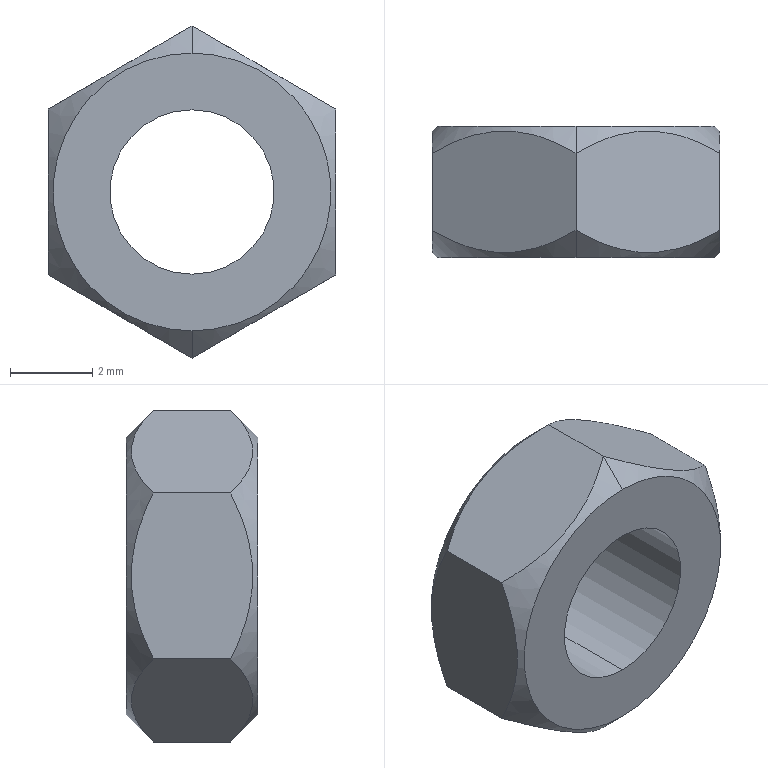Part | SolidWorks | features Extrusion 1, ICE 1, RevCut 1 | 1 solid | 14 faces | box 7 x 3.2 x 8.083 mm | volume 93.048 mm3 | plane 8 | cone 4 | cylinder 2 | commonest cylinder face diameters 4 x2
STEP:
#1=CARTESIAN_POINT('',(0.,0.,-2.));
#2=VERTEX_POINT('',#1);
#3=CARTESIAN_POINT('',(0.,0.,2.));
#4=VERTEX_POINT('',#3);
#5=CARTESIAN_POINT('',(0.,0.,0.));
#6=DIRECTION('',(0.,1.,0.));
#7=DIRECTION('',(0.,0.,1.));
#8=AXIS2_PLACEMENT_3D('',#5,#6,#7);
#9=CIRCLE('',#8,2.);
#10=EDGE_CURVE('',#2,#4,#9,.T.);
#11=ORIENTED_EDGE('',*,*,#10,.F.);
#12=CARTESIAN_POINT('',(0.,3.2,-2.));
#13=VERTEX_POINT('',#12);
#14=CARTESIAN_POINT('',(0.,0.,-2.));
#15=DIRECTION('',(0.,1.,0.));
#16=VECTOR('',#15,1000.);
#17=LINE('',#14,#16);
#18=EDGE_CURVE('',#2,#13,#17,.T.);
#19=ORIENTED_EDGE('',*,*,#18,.T.);
#20=CARTESIAN_POINT('',(0.,3.2,2.));
#21=VERTEX_POINT('',#20);
#22=CARTESIAN_POINT('',(0.,3.2,0.));
#23=DIRECTION('',(0.,1.,0.));
#24=DIRECTION('',(0.,0.,1.));
#25=AXIS2_PLACEMENT_3D('',#22,#23,#24);
#26=CIRCLE('',#25,2.);
#27=EDGE_CURVE('',#13,#21,#26,.T.);
#28=ORIENTED_EDGE('',*,*,#27,.T.);
#29=CARTESIAN_POINT('',(0.,0.,2.));
#30=DIRECTION('',(0.,1.,0.));
#31=VECTOR('',#30,1000.);
#32=LINE('',#29,#31);
#33=EDGE_CURVE('',#4,#21,#32,.T.);
#34=ORIENTED_EDGE('',*,*,#33,.F.);
#35=EDGE_LOOP('',(#11,#19,#28,#34));
#36=FACE_OUTER_BOUND('',#35,.T.);
#37=CARTESIAN_POINT('',(0.,0.,0.));
#38=DIRECTION('',(0.,1.,0.));
#39=DIRECTION('',(0.,0.,1.));
#40=AXIS2_PLACEMENT_3D('',#37,#38,#39);
#41=CYLINDRICAL_SURFACE('',#40,2.);
#42=ADVANCED_FACE('',(#36),#41,.F.);
#43=CARTESIAN_POINT('',(0.,3.2,-3.381));
#44=VERTEX_POINT('',#43);
#45=CARTESIAN_POINT('',(0.,3.2,3.381));
#46=VERTEX_POINT('',#45);
#47=CARTESIAN_POINT('',(0.,3.2,0.));
#48=DIRECTION('',(0.,-1.,0.));
#49=DIRECTION('',(0.,0.,-1.));
#50=AXIS2_PLACEMENT_3D('',#47,#48,#49);
#51=CIRCLE('',#50,3.381);
#52=EDGE_CURVE('',#44,#46,#51,.T.);
#53=ORIENTED_EDGE('',*,*,#52,.T.);
#54=CARTESIAN_POINT('',(0.,2.54,4.041));
#55=VERTEX_POINT('',#54);
#56=CARTESIAN_POINT('',(0.,3.2,3.381));
#57=DIRECTION('',(0.,-0.7071,0.7071));
#58=VECTOR('',#57,1000.);
#59=LINE('',#56,#58);
#60=EDGE_CURVE('',#46,#55,#59,.T.);
#61=ORIENTED_EDGE('',*,*,#60,.T.);
#62=CARTESIAN_POINT('',(3.5,2.54,2.021));
#63=VERTEX_POINT('',#62);
#64=CARTESIAN_POINT('',(3.5,2.54,2.021));
#65=CARTESIAN_POINT('',(3.227,2.698,2.179));
#66=CARTESIAN_POINT('',(2.947,2.832,2.34));
#67=CARTESIAN_POINT('',(2.512,2.976,2.591));
#68=CARTESIAN_POINT('',(2.365,3.014,2.676));
#69=CARTESIAN_POINT('',(2.064,3.067,2.85));
#70=CARTESIAN_POINT('',(1.909,3.081,2.939));
#71=CARTESIAN_POINT('',(1.451,3.082,3.204));
#72=CARTESIAN_POINT('',(1.151,3.029,3.377));
#73=CARTESIAN_POINT('',(0.5583,2.835,3.719));
#74=CARTESIAN_POINT('',(0.2751,2.699,3.883));
#75=CARTESIAN_POINT('',(0.,2.54,4.041));
#76=B_SPLINE_CURVE_WITH_KNOTS('',3,(#64,#65,#66,#67,#68,#69,#70,#71,#72,#73,#74,#75),.UNSPECIFIED.,.F.,.F.,(4,2,2,2,2,4),(0.000000254,0.001044,0.001566,0.002088,0.003131,0.004175),.UNSPECIFIED.);
#77=EDGE_CURVE('',#63,#55,#76,.T.);
#78=ORIENTED_EDGE('',*,*,#77,.F.);
#79=CARTESIAN_POINT('',(3.5,2.54,-2.021));
#80=VERTEX_POINT('',#79);
#81=CARTESIAN_POINT('',(3.5,2.54,-2.021));
#82=CARTESIAN_POINT('',(3.5,2.618,-1.864));
#83=CARTESIAN_POINT('',(3.5,2.691,-1.705));
#84=CARTESIAN_POINT('',(3.5,2.823,-1.378));
#85=CARTESIAN_POINT('',(3.5,2.882,-1.21));
#86=CARTESIAN_POINT('',(3.5,3.026,-0.7022));
#87=CARTESIAN_POINT('',(3.5,3.081,-0.357));
#88=CARTESIAN_POINT('',(3.5,3.082,0.1745));
#89=CARTESIAN_POINT('',(3.5,3.068,0.3526));
#90=CARTESIAN_POINT('',(3.5,3.016,0.7001));
#91=CARTESIAN_POINT('',(3.5,2.978,0.871));
#92=CARTESIAN_POINT('',(3.5,2.834,1.377));
#93=CARTESIAN_POINT('',(3.5,2.697,1.707));
#94=CARTESIAN_POINT('',(3.5,2.54,2.021));
#95=B_SPLINE_CURVE_WITH_KNOTS('',3,(#81,#82,#83,#84,#85,#86,#87,#88,#89,#90,#91,#92,#93,#94),.UNSPECIFIED.,.F.,.F.,(4,2,2,2,2,2,4),(0.005098,0.005624,0.00615,0.007203,0.00773,0.008256,0.009309),.UNSPECIFIED.);
#96=EDGE_CURVE('',#80,#63,#95,.T.);
#97=ORIENTED_EDGE('',*,*,#96,.F.);
#98=CARTESIAN_POINT('',(0.,2.54,-4.041));
#99=VERTEX_POINT('',#98);
#100=CARTESIAN_POINT('',(0.,2.54,-4.041));
#101=CARTESIAN_POINT('',(0.2735,2.698,-3.884));
#102=CARTESIAN_POINT('',(0.5531,2.832,-3.722));
#103=CARTESIAN_POINT('',(0.9875,2.976,-3.471));
#104=CARTESIAN_POINT('',(1.135,3.014,-3.386));
#105=CARTESIAN_POINT('',(1.436,3.067,-3.212));
#106=CARTESIAN_POINT('',(1.591,3.081,-3.123));
#107=CARTESIAN_POINT('',(2.049,3.082,-2.858));
#108=CARTESIAN_POINT('',(2.349,3.029,-2.685));
#109=CARTESIAN_POINT('',(2.942,2.835,-2.343));
#110=CARTESIAN_POINT('',(3.225,2.699,-2.18));
#111=CARTESIAN_POINT('',(3.5,2.54,-2.021));
#112=B_SPLINE_CURVE_WITH_KNOTS('',3,(#100,#101,#102,#103,#104,#105,#106,#107,#108,#109,#110,#111),.UNSPECIFIED.,.F.,.F.,(4,2,2,2,2,4),(0.000000254,0.001044,0.001566,0.002088,0.003131,0.004175),.UNSPECIFIED.);
#113=EDGE_CURVE('',#99,#80,#112,.T.);
#114=ORIENTED_EDGE('',*,*,#113,.F.);
#115=CARTESIAN_POINT('',(0.,3.2,-3.381));
#116=DIRECTION('',(0.,-0.7071,-0.7071));
#117=VECTOR('',#116,1000.);
#118=LINE('',#115,#117);
#119=EDGE_CURVE('',#44,#99,#118,.T.);
#120=ORIENTED_EDGE('',*,*,#119,.F.);
#121=EDGE_LOOP('',(#53,#61,#78,#97,#114,#120));
#122=FACE_OUTER_BOUND('',#121,.T.);
#123=CARTESIAN_POINT('',(0.,3.2,0.));
#124=DIRECTION('',(0.,-1.,0.));
#125=DIRECTION('',(0.,0.,-1.));
#126=AXIS2_PLACEMENT_3D('',#123,#124,#125);
#127=CONICAL_SURFACE('',#126,3.381,0.7854);
#128=ADVANCED_FACE('',(#122),#127,.T.);
#129=CARTESIAN_POINT('',(0.,0.,-3.381));
#130=VERTEX_POINT('',#129);
#131=CARTESIAN_POINT('',(0.,0.,3.381));
#132=VERTEX_POINT('',#131);
#133=CARTESIAN_POINT('',(0.,0.,0.));
#134=DIRECTION('',(0.,-1.,0.));
#135=DIRECTION('',(0.,0.,-1.));
#136=AXIS2_PLACEMENT_3D('',#133,#134,#135);
#137=CIRCLE('',#136,3.381);
#138=EDGE_CURVE('',#130,#132,#137,.T.);
#139=ORIENTED_EDGE('',*,*,#138,.F.);
#140=CARTESIAN_POINT('',(0.,0.66,-4.041));
#141=VERTEX_POINT('',#140);
#142=CARTESIAN_POINT('',(0.,0.66,-4.041));
#143=DIRECTION('',(0.,0.7071,-0.7071));
#144=VECTOR('',#143,1000.);
#145=LINE('',#142,#144);
#146=EDGE_CURVE('',#130,#141,#145,.T.);
#147=ORIENTED_EDGE('',*,*,#146,.T.);
#148=CARTESIAN_POINT('',(3.5,0.66,-2.021));
#149=VERTEX_POINT('',#148);
#150=CARTESIAN_POINT('',(3.5,0.66,-2.021));
#151=CARTESIAN_POINT('',(3.227,0.5021,-2.179));
#152=CARTESIAN_POINT('',(2.947,0.3679,-2.34));
#153=CARTESIAN_POINT('',(2.512,0.224,-2.591));
#154=CARTESIAN_POINT('',(2.365,0.1858,-2.676));
#155=CARTESIAN_POINT('',(2.064,0.1331,-2.85));
#156=CARTESIAN_POINT('',(1.909,0.1189,-2.939));
#157=CARTESIAN_POINT('',(1.451,0.1178,-3.204));
#158=CARTESIAN_POINT('',(1.151,0.1712,-3.377));
#159=CARTESIAN_POINT('',(0.5583,0.365,-3.719));
#160=CARTESIAN_POINT('',(0.2751,0.5012,-3.883));
#161=CARTESIAN_POINT('',(0.,0.66,-4.041));
#162=B_SPLINE_CURVE_WITH_KNOTS('',3,(#150,#151,#152,#153,#154,#155,#156,#157,#158,#159,#160,#161),.UNSPECIFIED.,.F.,.F.,(4,2,2,2,2,4),(0.000000254,0.001044,0.001566,0.002088,0.003131,0.004175),.UNSPECIFIED.);
#163=EDGE_CURVE('',#149,#141,#162,.T.);
#164=ORIENTED_EDGE('',*,*,#163,.F.);
#165=CARTESIAN_POINT('',(3.5,0.66,2.021));
#166=VERTEX_POINT('',#165);
#167=CARTESIAN_POINT('',(3.5,0.66,2.021));
#168=CARTESIAN_POINT('',(3.5,0.5818,1.864));
#169=CARTESIAN_POINT('',(3.5,0.5088,1.705));
#170=CARTESIAN_POINT('',(3.5,0.377,1.378));
#171=CARTESIAN_POINT('',(3.5,0.3181,1.21));
#172=CARTESIAN_POINT('',(3.5,0.1735,0.7022));
#173=CARTESIAN_POINT('',(3.5,0.1188,0.357));
#174=CARTESIAN_POINT('',(3.5,0.1184,-0.1745));
#175=CARTESIAN_POINT('',(3.5,0.1321,-0.3526));
#176=CARTESIAN_POINT('',(3.5,0.1837,-0.7001));
#177=CARTESIAN_POINT('',(3.5,0.2217,-0.871));
#178=CARTESIAN_POINT('',(3.5,0.3657,-1.377));
#179=CARTESIAN_POINT('',(3.5,0.5031,-1.707));
#180=CARTESIAN_POINT('',(3.5,0.66,-2.021));
#181=B_SPLINE_CURVE_WITH_KNOTS('',3,(#167,#168,#169,#170,#171,#172,#173,#174,#175,#176,#177,#178,#179,#180),.UNSPECIFIED.,.F.,.F.,(4,2,2,2,2,2,4),(0.005098,0.005624,0.00615,0.007203,0.00773,0.008256,0.009309),.UNSPECIFIED.);
#182=EDGE_CURVE('',#166,#149,#181,.T.);
#183=ORIENTED_EDGE('',*,*,#182,.F.);
#184=CARTESIAN_POINT('',(0.,0.66,4.041));
#185=VERTEX_POINT('',#184);
#186=CARTESIAN_POINT('',(0.,0.66,4.041));
#187=CARTESIAN_POINT('',(0.2735,0.5021,3.884));
#188=CARTESIAN_POINT('',(0.5531,0.3679,3.722));
#189=CARTESIAN_POINT('',(0.9875,0.224,3.471));
#190=CARTESIAN_POINT('',(1.135,0.1858,3.386));
#191=CARTESIAN_POINT('',(1.436,0.1331,3.212));
#192=CARTESIAN_POINT('',(1.591,0.1189,3.123));
#193=CARTESIAN_POINT('',(2.049,0.1178,2.858));
#194=CARTESIAN_POINT('',(2.349,0.1712,2.685));
#195=CARTESIAN_POINT('',(2.942,0.365,2.343));
#196=CARTESIAN_POINT('',(3.225,0.5012,2.18));
#197=CARTESIAN_POINT('',(3.5,0.66,2.021));
#198=B_SPLINE_CURVE_WITH_KNOTS('',3,(#186,#187,#188,#189,#190,#191,#192,#193,#194,#195,#196,#197),.UNSPECIFIED.,.F.,.F.,(4,2,2,2,2,4),(0.000000254,0.001044,0.001566,0.002088,0.003131,0.004175),.UNSPECIFIED.);
#199=EDGE_CURVE('',#185,#166,#198,.T.);
#200=ORIENTED_EDGE('',*,*,#199,.F.);
#201=CARTESIAN_POINT('',(0.,0.66,4.041));
#202=DIRECTION('',(0.,0.7071,0.7071));
#203=VECTOR('',#202,1000.);
#204=LINE('',#201,#203);
#205=EDGE_CURVE('',#132,#185,#204,.T.);
#206=ORIENTED_EDGE('',*,*,#205,.F.);
#207=EDGE_LOOP('',(#139,#147,#164,#183,#200,#206));
#208=FACE_OUTER_BOUND('',#207,.T.);
#209=CARTESIAN_POINT('',(0.,0.66,0.));
#210=DIRECTION('',(0.,1.,0.));
#211=DIRECTION('',(0.,0.,1.));
#212=AXIS2_PLACEMENT_3D('',#209,#210,#211);
#213=CONICAL_SURFACE('',#212,4.041,0.7854);
#214=ADVANCED_FACE('',(#208),#213,.T.);
#215=CARTESIAN_POINT('',(0.,0.,0.));
#216=DIRECTION('',(0.,1.,0.));
#217=DIRECTION('',(0.,0.,1.));
#218=AXIS2_PLACEMENT_3D('',#215,#216,#217);
#219=CIRCLE('',#218,2.);
#220=EDGE_CURVE('',#4,#2,#219,.T.);
#221=ORIENTED_EDGE('',*,*,#220,.T.);
#222=ORIENTED_EDGE('',*,*,#10,.T.);
#223=EDGE_LOOP('',(#221,#222));
#224=FACE_BOUND('',#223,.T.);
#225=CARTESIAN_POINT('',(0.,0.,0.));
#226=DIRECTION('',(0.,-1.,0.));
#227=DIRECTION('',(0.,0.,-1.));
#228=AXIS2_PLACEMENT_3D('',#225,#226,#227);
#229=CIRCLE('',#228,3.381);
#230=EDGE_CURVE('',#132,#130,#229,.T.);
#231=ORIENTED_EDGE('',*,*,#230,.T.);
#232=ORIENTED_EDGE('',*,*,#138,.T.);
#233=EDGE_LOOP('',(#231,#232));
#234=FACE_OUTER_BOUND('',#233,.T.);
#235=CARTESIAN_POINT('',(0.,0.,0.));
#236=DIRECTION('',(0.,1.,0.));
#237=DIRECTION('',(0.,0.,1.));
#238=AXIS2_PLACEMENT_3D('',#235,#236,#237);
#239=PLANE('',#238);
#240=ADVANCED_FACE('',(#224,#234),#239,.F.);
#241=ORIENTED_EDGE('',*,*,#146,.F.);
#242=ORIENTED_EDGE('',*,*,#230,.F.);
#243=ORIENTED_EDGE('',*,*,#205,.T.);
#244=CARTESIAN_POINT('',(-3.5,0.66,2.021));
#245=VERTEX_POINT('',#244);
#246=CARTESIAN_POINT('',(-3.5,0.66,2.021));
#247=CARTESIAN_POINT('',(-3.227,0.5021,2.179));
#248=CARTESIAN_POINT('',(-2.947,0.3679,2.34));
#249=CARTESIAN_POINT('',(-2.512,0.224,2.591));
#250=CARTESIAN_POINT('',(-2.365,0.1858,2.676));
#251=CARTESIAN_POINT('',(-2.064,0.1331,2.85));
#252=CARTESIAN_POINT('',(-1.909,0.1189,2.939));
#253=CARTESIAN_POINT('',(-1.451,0.1178,3.204));
#254=CARTESIAN_POINT('',(-1.151,0.1712,3.377));
#255=CARTESIAN_POINT('',(-0.5583,0.365,3.719));
#256=CARTESIAN_POINT('',(-0.2751,0.5012,3.883));
#257=CARTESIAN_POINT('',(0.,0.66,4.041));
#258=B_SPLINE_CURVE_WITH_KNOTS('',3,(#246,#247,#248,#249,#250,#251,#252,#253,#254,#255,#256,#257),.UNSPECIFIED.,.F.,.F.,(4,2,2,2,2,4),(0.000000254,0.001044,0.001566,0.002088,0.003131,0.004175),.UNSPECIFIED.);
#259=EDGE_CURVE('',#245,#185,#258,.T.);
#260=ORIENTED_EDGE('',*,*,#259,.F.);
#261=CARTESIAN_POINT('',(-3.5,0.66,-2.021));
#262=VERTEX_POINT('',#261);
#263=CARTESIAN_POINT('',(-3.5,0.66,-2.021));
#264=CARTESIAN_POINT('',(-3.5,0.5818,-1.864));
#265=CARTESIAN_POINT('',(-3.5,0.5088,-1.705));
#266=CARTESIAN_POINT('',(-3.5,0.377,-1.378));
#267=CARTESIAN_POINT('',(-3.5,0.3181,-1.21));
#268=CARTESIAN_POINT('',(-3.5,0.1735,-0.7022));
#269=CARTESIAN_POINT('',(-3.5,0.1188,-0.357));
#270=CARTESIAN_POINT('',(-3.5,0.1184,0.1745));
#271=CARTESIAN_POINT('',(-3.5,0.1321,0.3526));
#272=CARTESIAN_POINT('',(-3.5,0.1837,0.7001));
#273=CARTESIAN_POINT('',(-3.5,0.2217,0.871));
#274=CARTESIAN_POINT('',(-3.5,0.3657,1.377));
#275=CARTESIAN_POINT('',(-3.5,0.5031,1.707));
#276=CARTESIAN_POINT('',(-3.5,0.66,2.021));
#277=B_SPLINE_CURVE_WITH_KNOTS('',3,(#263,#264,#265,#266,#267,#268,#269,#270,#271,#272,#273,#274,#275,#276),.UNSPECIFIED.,.F.,.F.,(4,2,2,2,2,2,4),(0.005098,0.005624,0.00615,0.007203,0.00773,0.008256,0.009309),.UNSPECIFIED.);
#278=EDGE_CURVE('',#262,#245,#277,.T.);
#279=ORIENTED_EDGE('',*,*,#278,.F.);
#280=CARTESIAN_POINT('',(0.,0.66,-4.041));
#281=CARTESIAN_POINT('',(-0.2735,0.5021,-3.884));
#282=CARTESIAN_POINT('',(-0.5531,0.3679,-3.722));
#283=CARTESIAN_POINT('',(-0.9875,0.224,-3.471));
#284=CARTESIAN_POINT('',(-1.135,0.1858,-3.386));
#285=CARTESIAN_POINT('',(-1.436,0.1331,-3.212));
#286=CARTESIAN_POINT('',(-1.591,0.1189,-3.123));
#287=CARTESIAN_POINT('',(-2.049,0.1178,-2.858));
#288=CARTESIAN_POINT('',(-2.349,0.1712,-2.685));
#289=CARTESIAN_POINT('',(-2.942,0.365,-2.343));
#290=CARTESIAN_POINT('',(-3.225,0.5012,-2.18));
#291=CARTESIAN_POINT('',(-3.5,0.66,-2.021));
#292=B_SPLINE_CURVE_WITH_KNOTS('',3,(#280,#281,#282,#283,#284,#285,#286,#287,#288,#289,#290,#291),.UNSPECIFIED.,.F.,.F.,(4,2,2,2,2,4),(0.000000254,0.001044,0.001566,0.002088,0.003131,0.004175),.UNSPECIFIED.);
#293=EDGE_CURVE('',#141,#262,#292,.T.);
#294=ORIENTED_EDGE('',*,*,#293,.F.);
#295=EDGE_LOOP('',(#241,#242,#243,#260,#279,#294));
#296=FACE_OUTER_BOUND('',#295,.T.);
#297=CARTESIAN_POINT('',(0.,0.66,0.));
#298=DIRECTION('',(0.,1.,0.));
#299=DIRECTION('',(0.,0.,1.));
#300=AXIS2_PLACEMENT_3D('',#297,#298,#299);
#301=CONICAL_SURFACE('',#300,4.041,0.7854);
#302=ADVANCED_FACE('',(#296),#301,.T.);
#303=CARTESIAN_POINT('',(0.,3.2,-4.041));
#304=DIRECTION('',(0.,-1.,0.));
#305=VECTOR('',#304,1000.);
#306=LINE('',#303,#305);
#307=EDGE_CURVE('',#99,#141,#306,.T.);
#308=ORIENTED_EDGE('',*,*,#307,.F.);
#309=ORIENTED_EDGE('',*,*,#113,.T.);
#310=CARTESIAN_POINT('',(3.5,3.2,-2.021));
#311=DIRECTION('',(0.,-1.,0.));
#312=VECTOR('',#311,1000.);
#313=LINE('',#310,#312);
#314=EDGE_CURVE('',#80,#149,#313,.T.);
#315=ORIENTED_EDGE('',*,*,#314,.T.);
#316=ORIENTED_EDGE('',*,*,#163,.T.);
#317=EDGE_LOOP('',(#308,#309,#315,#316));
#318=FACE_OUTER_BOUND('',#317,.T.);
#319=CARTESIAN_POINT('',(3.5,3.2,-2.021));
#320=DIRECTION('',(-0.5,0.,0.866));
#321=DIRECTION('',(0.866,0.,0.5));
#322=AXIS2_PLACEMENT_3D('',#319,#320,#321);
#323=PLANE('',#322);
#324=ADVANCED_FACE('',(#318),#323,.F.);
#325=CARTESIAN_POINT('',(-3.5,2.54,-2.021));
#326=VERTEX_POINT('',#325);
#327=CARTESIAN_POINT('',(-3.5,3.2,-2.021));
#328=DIRECTION('',(0.,-1.,0.));
#329=VECTOR('',#328,1000.);
#330=LINE('',#327,#329);
#331=EDGE_CURVE('',#326,#262,#330,.T.);
#332=ORIENTED_EDGE('',*,*,#331,.F.);
#333=CARTESIAN_POINT('',(-3.5,2.54,-2.021));
#334=CARTESIAN_POINT('',(-3.227,2.698,-2.179));
#335=CARTESIAN_POINT('',(-2.947,2.832,-2.34));
#336=CARTESIAN_POINT('',(-2.512,2.976,-2.591));
#337=CARTESIAN_POINT('',(-2.365,3.014,-2.676));
#338=CARTESIAN_POINT('',(-2.064,3.067,-2.85));
#339=CARTESIAN_POINT('',(-1.909,3.081,-2.939));
#340=CARTESIAN_POINT('',(-1.451,3.082,-3.204));
#341=CARTESIAN_POINT('',(-1.151,3.029,-3.377));
#342=CARTESIAN_POINT('',(-0.5583,2.835,-3.719));
#343=CARTESIAN_POINT('',(-0.2751,2.699,-3.883));
#344=CARTESIAN_POINT('',(0.,2.54,-4.041));
#345=B_SPLINE_CURVE_WITH_KNOTS('',3,(#333,#334,#335,#336,#337,#338,#339,#340,#341,#342,#343,#344),.UNSPECIFIED.,.F.,.F.,(4,2,2,2,2,4),(0.000000254,0.001044,0.001566,0.002088,0.003131,0.004175),.UNSPECIFIED.);
#346=EDGE_CURVE('',#326,#99,#345,.T.);
#347=ORIENTED_EDGE('',*,*,#346,.T.);
#348=ORIENTED_EDGE('',*,*,#307,.T.);
#349=ORIENTED_EDGE('',*,*,#293,.T.);
#350=EDGE_LOOP('',(#332,#347,#348,#349));
#351=FACE_OUTER_BOUND('',#350,.T.);
#352=CARTESIAN_POINT('',(0.,3.2,-4.041));
#353=DIRECTION('',(0.5,0.,0.866));
#354=DIRECTION('',(0.866,0.,-0.5));
#355=AXIS2_PLACEMENT_3D('',#352,#353,#354);
#356=PLANE('',#355);
#357=ADVANCED_FACE('',(#351),#356,.F.);
#358=CARTESIAN_POINT('',(-3.5,2.54,2.021));
#359=VERTEX_POINT('',#358);
#360=CARTESIAN_POINT('',(-3.5,3.2,2.021));
#361=DIRECTION('',(0.,-1.,0.));
#362=VECTOR('',#361,1000.);
#363=LINE('',#360,#362);
#364=EDGE_CURVE('',#359,#245,#363,.T.);
#365=ORIENTED_EDGE('',*,*,#364,.F.);
#366=CARTESIAN_POINT('',(-3.5,2.54,2.021));
#367=CARTESIAN_POINT('',(-3.5,2.618,1.864));
#368=CARTESIAN_POINT('',(-3.5,2.691,1.705));
#369=CARTESIAN_POINT('',(-3.5,2.823,1.378));
#370=CARTESIAN_POINT('',(-3.5,2.882,1.21));
#371=CARTESIAN_POINT('',(-3.5,3.026,0.7022));
#372=CARTESIAN_POINT('',(-3.5,3.081,0.357));
#373=CARTESIAN_POINT('',(-3.5,3.082,-0.1745));
#374=CARTESIAN_POINT('',(-3.5,3.068,-0.3526));
#375=CARTESIAN_POINT('',(-3.5,3.016,-0.7001));
#376=CARTESIAN_POINT('',(-3.5,2.978,-0.871));
#377=CARTESIAN_POINT('',(-3.5,2.834,-1.377));
#378=CARTESIAN_POINT('',(-3.5,2.697,-1.707));
#379=CARTESIAN_POINT('',(-3.5,2.54,-2.021));
#380=B_SPLINE_CURVE_WITH_KNOTS('',3,(#366,#367,#368,#369,#370,#371,#372,#373,#374,#375,#376,#377,#378,#379),.UNSPECIFIED.,.F.,.F.,(4,2,2,2,2,2,4),(0.005098,0.005624,0.00615,0.007203,0.00773,0.008256,0.009309),.UNSPECIFIED.);
#381=EDGE_CURVE('',#359,#326,#380,.T.);
#382=ORIENTED_EDGE('',*,*,#381,.T.);
#383=ORIENTED_EDGE('',*,*,#331,.T.);
#384=ORIENTED_EDGE('',*,*,#278,.T.);
#385=EDGE_LOOP('',(#365,#382,#383,#384));
#386=FACE_OUTER_BOUND('',#385,.T.);
#387=CARTESIAN_POINT('',(-3.5,3.2,-2.021));
#388=DIRECTION('',(1.,0.,0.));
#389=DIRECTION('',(0.,0.,-1.));
#390=AXIS2_PLACEMENT_3D('',#387,#388,#389);
#391=PLANE('',#390);
#392=ADVANCED_FACE('',(#386),#391,.F.);
#393=CARTESIAN_POINT('',(0.,3.2,4.041));
#394=DIRECTION('',(0.,-1.,0.));
#395=VECTOR('',#394,1000.);
#396=LINE('',#393,#395);
#397=EDGE_CURVE('',#55,#185,#396,.T.);
#398=ORIENTED_EDGE('',*,*,#397,.F.);
#399=CARTESIAN_POINT('',(0.,2.54,4.041));
#400=CARTESIAN_POINT('',(-0.2735,2.698,3.884));
#401=CARTESIAN_POINT('',(-0.5531,2.832,3.722));
#402=CARTESIAN_POINT('',(-0.9875,2.976,3.471));
#403=CARTESIAN_POINT('',(-1.135,3.014,3.386));
#404=CARTESIAN_POINT('',(-1.436,3.067,3.212));
#405=CARTESIAN_POINT('',(-1.591,3.081,3.123));
#406=CARTESIAN_POINT('',(-2.049,3.082,2.858));
#407=CARTESIAN_POINT('',(-2.349,3.029,2.685));
#408=CARTESIAN_POINT('',(-2.942,2.835,2.343));
#409=CARTESIAN_POINT('',(-3.225,2.699,2.18));
#410=CARTESIAN_POINT('',(-3.5,2.54,2.021));
#411=B_SPLINE_CURVE_WITH_KNOTS('',3,(#399,#400,#401,#402,#403,#404,#405,#406,#407,#408,#409,#410),.UNSPECIFIED.,.F.,.F.,(4,2,2,2,2,4),(0.000000254,0.001044,0.001566,0.002088,0.003131,0.004175),.UNSPECIFIED.);
#412=EDGE_CURVE('',#55,#359,#411,.T.);
#413=ORIENTED_EDGE('',*,*,#412,.T.);
#414=ORIENTED_EDGE('',*,*,#364,.T.);
#415=ORIENTED_EDGE('',*,*,#259,.T.);
#416=EDGE_LOOP('',(#398,#413,#414,#415));
#417=FACE_OUTER_BOUND('',#416,.T.);
#418=CARTESIAN_POINT('',(-3.5,3.2,2.021));
#419=DIRECTION('',(0.5,0.,-0.866));
#420=DIRECTION('',(-0.866,0.,-0.5));
#421=AXIS2_PLACEMENT_3D('',#418,#419,#420);
#422=PLANE('',#421);
#423=ADVANCED_FACE('',(#417),#422,.F.);
#424=CARTESIAN_POINT('',(3.5,3.2,2.021));
#425=DIRECTION('',(0.,-1.,0.));
#426=VECTOR('',#425,1000.);
#427=LINE('',#424,#426);
#428=EDGE_CURVE('',#63,#166,#427,.T.);
#429=ORIENTED_EDGE('',*,*,#428,.F.);
#430=ORIENTED_EDGE('',*,*,#77,.T.);
#431=ORIENTED_EDGE('',*,*,#397,.T.);
#432=ORIENTED_EDGE('',*,*,#199,.T.);
#433=EDGE_LOOP('',(#429,#430,#431,#432));
#434=FACE_OUTER_BOUND('',#433,.T.);
#435=CARTESIAN_POINT('',(0.,3.2,4.041));
#436=DIRECTION('',(-0.5,0.,-0.866));
#437=DIRECTION('',(-0.866,0.,0.5));
#438=AXIS2_PLACEMENT_3D('',#435,#436,#437);
#439=PLANE('',#438);
#440=ADVANCED_FACE('',(#434),#439,.F.);
#441=ORIENTED_EDGE('',*,*,#314,.F.);
#442=ORIENTED_EDGE('',*,*,#96,.T.);
#443=ORIENTED_EDGE('',*,*,#428,.T.);
#444=ORIENTED_EDGE('',*,*,#182,.T.);
#445=EDGE_LOOP('',(#441,#442,#443,#444));
#446=FACE_OUTER_BOUND('',#445,.T.);
#447=CARTESIAN_POINT('',(3.5,3.2,2.021));
#448=DIRECTION('',(-1.,0.,0.));
#449=DIRECTION('',(0.,0.,1.));
#450=AXIS2_PLACEMENT_3D('',#447,#448,#449);
#451=PLANE('',#450);
#452=ADVANCED_FACE('',(#446),#451,.F.);
#453=ORIENTED_EDGE('',*,*,#60,.F.);
#454=CARTESIAN_POINT('',(0.,3.2,0.));
#455=DIRECTION('',(0.,-1.,0.));
#456=DIRECTION('',(0.,0.,-1.));
#457=AXIS2_PLACEMENT_3D('',#454,#455,#456);
#458=CIRCLE('',#457,3.381);
#459=EDGE_CURVE('',#46,#44,#458,.T.);
#460=ORIENTED_EDGE('',*,*,#459,.T.);
#461=ORIENTED_EDGE('',*,*,#119,.T.);
#462=ORIENTED_EDGE('',*,*,#346,.F.);
#463=ORIENTED_EDGE('',*,*,#381,.F.);
#464=ORIENTED_EDGE('',*,*,#412,.F.);
#465=EDGE_LOOP('',(#453,#460,#461,#462,#463,#464));
#466=FACE_OUTER_BOUND('',#465,.T.);
#467=CARTESIAN_POINT('',(0.,3.2,0.));
#468=DIRECTION('',(0.,-1.,0.));
#469=DIRECTION('',(0.,0.,-1.));
#470=AXIS2_PLACEMENT_3D('',#467,#468,#469);
#471=CONICAL_SURFACE('',#470,3.381,0.7854);
#472=ADVANCED_FACE('',(#466),#471,.T.);
#473=CARTESIAN_POINT('',(0.,3.2,0.));
#474=DIRECTION('',(0.,1.,0.));
#475=DIRECTION('',(0.,0.,1.));
#476=AXIS2_PLACEMENT_3D('',#473,#474,#475);
#477=CIRCLE('',#476,2.);
#478=EDGE_CURVE('',#21,#13,#477,.T.);
#479=ORIENTED_EDGE('',*,*,#478,.F.);
#480=ORIENTED_EDGE('',*,*,#27,.F.);
#481=EDGE_LOOP('',(#479,#480));
#482=FACE_BOUND('',#481,.T.);
#483=ORIENTED_EDGE('',*,*,#52,.F.);
#484=ORIENTED_EDGE('',*,*,#459,.F.);
#485=EDGE_LOOP('',(#483,#484));
#486=FACE_OUTER_BOUND('',#485,.T.);
#487=CARTESIAN_POINT('',(0.,3.2,0.));
#488=DIRECTION('',(0.,1.,0.));
#489=DIRECTION('',(0.,0.,1.));
#490=AXIS2_PLACEMENT_3D('',#487,#488,#489);
#491=PLANE('',#490);
#492=ADVANCED_FACE('',(#482,#486),#491,.T.);
#493=ORIENTED_EDGE('',*,*,#18,.F.);
#494=ORIENTED_EDGE('',*,*,#220,.F.);
#495=ORIENTED_EDGE('',*,*,#33,.T.);
#496=ORIENTED_EDGE('',*,*,#478,.T.);
#497=EDGE_LOOP('',(#493,#494,#495,#496));
#498=FACE_OUTER_BOUND('',#497,.T.);
#499=CARTESIAN_POINT('',(0.,0.,0.));
#500=DIRECTION('',(0.,1.,0.));
#501=DIRECTION('',(0.,0.,1.));
#502=AXIS2_PLACEMENT_3D('',#499,#500,#501);
#503=CYLINDRICAL_SURFACE('',#502,2.);
#504=ADVANCED_FACE('',(#498),#503,.F.);
#505=CLOSED_SHELL('',(#42,#128,#214,#240,#302,#324,#357,#392,#423,#440,#452,#472,#492,#504));
#506=MANIFOLD_SOLID_BREP('',#505);
#507=CARTESIAN_POINT('',(0.,0.,0.));
#508=DIRECTION('',(0.,0.,1.));
#509=DIRECTION('',(1.,0.,0.));
#510=AXIS2_PLACEMENT_3D('',#507,#508,#509);
#511=(LENGTH_UNIT()NAMED_UNIT(*)SI_UNIT(.MILLI.,.METRE.));
#512=UNCERTAINTY_MEASURE_WITH_UNIT(LENGTH_MEASURE(0.00001),#511,'','');
#513=(NAMED_UNIT(*)PLANE_ANGLE_UNIT()SI_UNIT($,.RADIAN.));
#514=(NAMED_UNIT(*)SI_UNIT($,.STERADIAN.)SOLID_ANGLE_UNIT());
#515=(GEOMETRIC_REPRESENTATION_CONTEXT(3)GLOBAL_UNCERTAINTY_ASSIGNED_CONTEXT((#512))GLOBAL_UNIT_ASSIGNED_CONTEXT((#511,#513,#514))REPRESENTATION_CONTEXT('',''));
#516=ADVANCED_BREP_SHAPE_REPRESENTATION('',(#506,#510),#515);